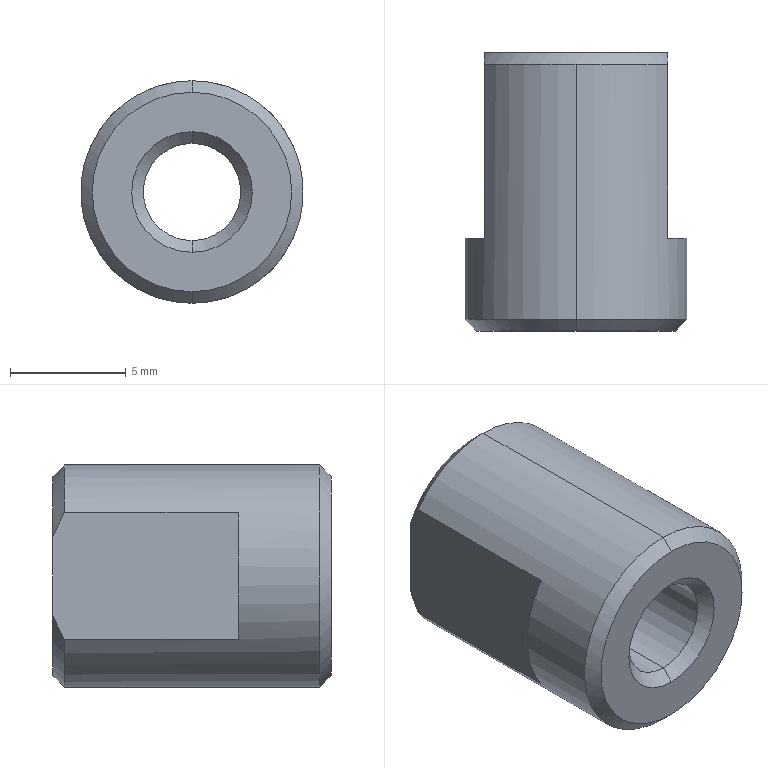Part | SolidWorks | features HoleWzd 1, ICE 1, Revolution 1 | 1 solid | 19 faces | box 9.6 x 12 x 9.6 mm | volume 642.366 mm3 | cone 9 | plane 6 | cylinder 4 | commonest cylinder face diameters 4.2 x2 9.6 x2
STEP:
#1=CARTESIAN_POINT('',(0.,11.5,-2.1));
#2=VERTEX_POINT('',#1);
#3=CARTESIAN_POINT('',(0.,11.5,2.1));
#4=VERTEX_POINT('',#3);
#5=CARTESIAN_POINT('',(0.,11.5,0.));
#6=DIRECTION('',(0.,1.,0.));
#7=DIRECTION('',(0.,0.,1.));
#8=AXIS2_PLACEMENT_3D('',#5,#6,#7);
#9=CIRCLE('',#8,2.1);
#10=EDGE_CURVE('',#2,#4,#9,.T.);
#11=ORIENTED_EDGE('',*,*,#10,.F.);
#12=CARTESIAN_POINT('',(0.,12.,-2.6));
#13=VERTEX_POINT('',#12);
#14=CARTESIAN_POINT('',(0.,12.,-2.6));
#15=DIRECTION('',(0.,0.7071,-0.7071));
#16=VECTOR('',#15,1000.);
#17=LINE('',#14,#16);
#18=EDGE_CURVE('',#2,#13,#17,.T.);
#19=ORIENTED_EDGE('',*,*,#18,.T.);
#20=CARTESIAN_POINT('',(0.,12.,2.6));
#21=VERTEX_POINT('',#20);
#22=CARTESIAN_POINT('',(0.,12.,0.));
#23=DIRECTION('',(0.,1.,0.));
#24=DIRECTION('',(0.,0.,1.));
#25=AXIS2_PLACEMENT_3D('',#22,#23,#24);
#26=CIRCLE('',#25,2.6);
#27=EDGE_CURVE('',#13,#21,#26,.T.);
#28=ORIENTED_EDGE('',*,*,#27,.T.);
#29=CARTESIAN_POINT('',(0.,12.,2.6));
#30=DIRECTION('',(0.,0.7071,0.7071));
#31=VECTOR('',#30,1000.);
#32=LINE('',#29,#31);
#33=EDGE_CURVE('',#4,#21,#32,.T.);
#34=ORIENTED_EDGE('',*,*,#33,.F.);
#35=EDGE_LOOP('',(#11,#19,#28,#34));
#36=FACE_OUTER_BOUND('',#35,.T.);
#37=CARTESIAN_POINT('',(0.,12.,0.));
#38=DIRECTION('',(0.,1.,0.));
#39=DIRECTION('',(0.,0.,1.));
#40=AXIS2_PLACEMENT_3D('',#37,#38,#39);
#41=CONICAL_SURFACE('',#40,2.6,0.7854);
#42=ADVANCED_FACE('',(#36),#41,.F.);
#43=CARTESIAN_POINT('',(0.,0.5,-2.1));
#44=VERTEX_POINT('',#43);
#45=CARTESIAN_POINT('',(0.,0.5,2.1));
#46=VERTEX_POINT('',#45);
#47=CARTESIAN_POINT('',(0.,0.5,0.));
#48=DIRECTION('',(0.,1.,0.));
#49=DIRECTION('',(0.,0.,1.));
#50=AXIS2_PLACEMENT_3D('',#47,#48,#49);
#51=CIRCLE('',#50,2.1);
#52=EDGE_CURVE('',#44,#46,#51,.T.);
#53=ORIENTED_EDGE('',*,*,#52,.F.);
#54=CARTESIAN_POINT('',(0.,12.,-2.1));
#55=DIRECTION('',(0.,1.,0.));
#56=VECTOR('',#55,1000.);
#57=LINE('',#54,#56);
#58=EDGE_CURVE('',#44,#2,#57,.T.);
#59=ORIENTED_EDGE('',*,*,#58,.T.);
#60=ORIENTED_EDGE('',*,*,#10,.T.);
#61=CARTESIAN_POINT('',(0.,12.,2.1));
#62=DIRECTION('',(0.,1.,0.));
#63=VECTOR('',#62,1000.);
#64=LINE('',#61,#63);
#65=EDGE_CURVE('',#46,#4,#64,.T.);
#66=ORIENTED_EDGE('',*,*,#65,.F.);
#67=EDGE_LOOP('',(#53,#59,#60,#66));
#68=FACE_OUTER_BOUND('',#67,.T.);
#69=CARTESIAN_POINT('',(0.,12.,0.));
#70=DIRECTION('',(0.,1.,0.));
#71=DIRECTION('',(0.,0.,1.));
#72=AXIS2_PLACEMENT_3D('',#69,#70,#71);
#73=CYLINDRICAL_SURFACE('',#72,2.1);
#74=ADVANCED_FACE('',(#68),#73,.F.);
#75=ORIENTED_EDGE('',*,*,#52,.T.);
#76=CARTESIAN_POINT('',(0.,0.,2.6));
#77=VERTEX_POINT('',#76);
#78=CARTESIAN_POINT('',(0.,0.5,2.1));
#79=DIRECTION('',(0.,-0.7071,0.7071));
#80=VECTOR('',#79,1000.);
#81=LINE('',#78,#80);
#82=EDGE_CURVE('',#46,#77,#81,.T.);
#83=ORIENTED_EDGE('',*,*,#82,.T.);
#84=CARTESIAN_POINT('',(0.,0.,-2.6));
#85=VERTEX_POINT('',#84);
#86=CARTESIAN_POINT('',(0.,0.,0.));
#87=DIRECTION('',(0.,1.,0.));
#88=DIRECTION('',(0.,0.,1.));
#89=AXIS2_PLACEMENT_3D('',#86,#87,#88);
#90=CIRCLE('',#89,2.6);
#91=EDGE_CURVE('',#85,#77,#90,.T.);
#92=ORIENTED_EDGE('',*,*,#91,.F.);
#93=CARTESIAN_POINT('',(0.,0.5,-2.1));
#94=DIRECTION('',(0.,-0.7071,-0.7071));
#95=VECTOR('',#94,1000.);
#96=LINE('',#93,#95);
#97=EDGE_CURVE('',#44,#85,#96,.T.);
#98=ORIENTED_EDGE('',*,*,#97,.F.);
#99=EDGE_LOOP('',(#75,#83,#92,#98));
#100=FACE_OUTER_BOUND('',#99,.T.);
#101=CARTESIAN_POINT('',(0.,0.5,0.));
#102=DIRECTION('',(0.,-1.,0.));
#103=DIRECTION('',(0.,0.,-1.));
#104=AXIS2_PLACEMENT_3D('',#101,#102,#103);
#105=CONICAL_SURFACE('',#104,2.1,0.7854);
#106=ADVANCED_FACE('',(#100),#105,.F.);
#107=CARTESIAN_POINT('',(0.,0.,-4.3));
#108=VERTEX_POINT('',#107);
#109=CARTESIAN_POINT('',(0.,0.,4.3));
#110=VERTEX_POINT('',#109);
#111=CARTESIAN_POINT('',(0.,0.,0.));
#112=DIRECTION('',(0.,-1.,0.));
#113=DIRECTION('',(0.,0.,-1.));
#114=AXIS2_PLACEMENT_3D('',#111,#112,#113);
#115=CIRCLE('',#114,4.3);
#116=EDGE_CURVE('',#108,#110,#115,.T.);
#117=ORIENTED_EDGE('',*,*,#116,.F.);
#118=CARTESIAN_POINT('',(0.,0.5,-4.8));
#119=VERTEX_POINT('',#118);
#120=CARTESIAN_POINT('',(0.,0.,-4.3));
#121=DIRECTION('',(0.,0.7071,-0.7071));
#122=VECTOR('',#121,1000.);
#123=LINE('',#120,#122);
#124=EDGE_CURVE('',#108,#119,#123,.T.);
#125=ORIENTED_EDGE('',*,*,#124,.T.);
#126=CARTESIAN_POINT('',(0.,0.5,4.8));
#127=VERTEX_POINT('',#126);
#128=CARTESIAN_POINT('',(0.,0.5,0.));
#129=DIRECTION('',(0.,-1.,0.));
#130=DIRECTION('',(0.,0.,-1.));
#131=AXIS2_PLACEMENT_3D('',#128,#129,#130);
#132=CIRCLE('',#131,4.8);
#133=EDGE_CURVE('',#119,#127,#132,.T.);
#134=ORIENTED_EDGE('',*,*,#133,.T.);
#135=CARTESIAN_POINT('',(0.,0.,4.3));
#136=DIRECTION('',(0.,0.7071,0.7071));
#137=VECTOR('',#136,1000.);
#138=LINE('',#135,#137);
#139=EDGE_CURVE('',#110,#127,#138,.T.);
#140=ORIENTED_EDGE('',*,*,#139,.F.);
#141=EDGE_LOOP('',(#117,#125,#134,#140));
#142=FACE_OUTER_BOUND('',#141,.T.);
#143=CARTESIAN_POINT('',(0.,0.,0.));
#144=DIRECTION('',(0.,1.,0.));
#145=DIRECTION('',(0.,0.,1.));
#146=AXIS2_PLACEMENT_3D('',#143,#144,#145);
#147=CONICAL_SURFACE('',#146,4.3,0.7854);
#148=ADVANCED_FACE('',(#142),#147,.T.);
#149=CARTESIAN_POINT('',(3.95,11.5,2.727));
#150=VERTEX_POINT('',#149);
#151=CARTESIAN_POINT('',(0.,11.5,4.8));
#152=VERTEX_POINT('',#151);
#153=CARTESIAN_POINT('',(0.,11.5,0.));
#154=DIRECTION('',(0.,-1.,0.));
#155=DIRECTION('',(0.,0.,-1.));
#156=AXIS2_PLACEMENT_3D('',#153,#154,#155);
#157=CIRCLE('',#156,4.8);
#158=EDGE_CURVE('',#150,#152,#157,.T.);
#159=ORIENTED_EDGE('',*,*,#158,.T.);
#160=CARTESIAN_POINT('',(0.,12.,4.8));
#161=DIRECTION('',(0.,-1.,0.));
#162=VECTOR('',#161,1000.);
#163=LINE('',#160,#162);
#164=EDGE_CURVE('',#152,#127,#163,.T.);
#165=ORIENTED_EDGE('',*,*,#164,.T.);
#166=ORIENTED_EDGE('',*,*,#133,.F.);
#167=CARTESIAN_POINT('',(0.,11.5,-4.8));
#168=VERTEX_POINT('',#167);
#169=CARTESIAN_POINT('',(0.,12.,-4.8));
#170=DIRECTION('',(0.,-1.,0.));
#171=VECTOR('',#170,1000.);
#172=LINE('',#169,#171);
#173=EDGE_CURVE('',#168,#119,#172,.T.);
#174=ORIENTED_EDGE('',*,*,#173,.F.);
#175=CARTESIAN_POINT('',(3.95,11.5,-2.727));
#176=VERTEX_POINT('',#175);
#177=CARTESIAN_POINT('',(0.,11.5,0.));
#178=DIRECTION('',(0.,-1.,0.));
#179=DIRECTION('',(0.,0.,-1.));
#180=AXIS2_PLACEMENT_3D('',#177,#178,#179);
#181=CIRCLE('',#180,4.8);
#182=EDGE_CURVE('',#168,#176,#181,.T.);
#183=ORIENTED_EDGE('',*,*,#182,.T.);
#184=CARTESIAN_POINT('',(3.95,4.,-2.727));
#185=VERTEX_POINT('',#184);
#186=CARTESIAN_POINT('',(3.95,12.,-2.727));
#187=DIRECTION('',(0.,1.,0.));
#188=VECTOR('',#187,1000.);
#189=LINE('',#186,#188);
#190=EDGE_CURVE('',#185,#176,#189,.T.);
#191=ORIENTED_EDGE('',*,*,#190,.F.);
#192=CARTESIAN_POINT('',(3.95,4.,2.727));
#193=VERTEX_POINT('',#192);
#194=CARTESIAN_POINT('',(0.,4.,0.));
#195=DIRECTION('',(0.,1.,0.));
#196=DIRECTION('',(0.,0.,-1.));
#197=AXIS2_PLACEMENT_3D('',#194,#195,#196);
#198=CIRCLE('',#197,4.8);
#199=EDGE_CURVE('',#193,#185,#198,.T.);
#200=ORIENTED_EDGE('',*,*,#199,.F.);
#201=CARTESIAN_POINT('',(3.95,12.,2.727));
#202=DIRECTION('',(0.,-1.,0.));
#203=VECTOR('',#202,1000.);
#204=LINE('',#201,#203);
#205=EDGE_CURVE('',#150,#193,#204,.T.);
#206=ORIENTED_EDGE('',*,*,#205,.F.);
#207=EDGE_LOOP('',(#159,#165,#166,#174,#183,#191,#200,#206));
#208=FACE_OUTER_BOUND('',#207,.T.);
#209=CARTESIAN_POINT('',(0.,12.,0.));
#210=DIRECTION('',(0.,-1.,0.));
#211=DIRECTION('',(0.,0.,-1.));
#212=AXIS2_PLACEMENT_3D('',#209,#210,#211);
#213=CYLINDRICAL_SURFACE('',#212,4.8);
#214=ADVANCED_FACE('',(#208),#213,.T.);
#215=CARTESIAN_POINT('',(-3.95,12.,-1.699));
#216=VERTEX_POINT('',#215);
#217=CARTESIAN_POINT('',(0.,12.,-4.3));
#218=VERTEX_POINT('',#217);
#219=CARTESIAN_POINT('',(0.,12.,0.));
#220=DIRECTION('',(0.,-1.,0.));
#221=DIRECTION('',(0.,0.,-1.));
#222=AXIS2_PLACEMENT_3D('',#219,#220,#221);
#223=CIRCLE('',#222,4.3);
#224=EDGE_CURVE('',#216,#218,#223,.T.);
#225=ORIENTED_EDGE('',*,*,#224,.T.);
#226=CARTESIAN_POINT('',(0.,11.5,-4.8));
#227=DIRECTION('',(0.,-0.7071,-0.7071));
#228=VECTOR('',#227,1000.);
#229=LINE('',#226,#228);
#230=EDGE_CURVE('',#218,#168,#229,.T.);
#231=ORIENTED_EDGE('',*,*,#230,.T.);
#232=CARTESIAN_POINT('',(-3.95,11.5,-2.727));
#233=VERTEX_POINT('',#232);
#234=CARTESIAN_POINT('',(0.,11.5,0.));
#235=DIRECTION('',(0.,-1.,0.));
#236=DIRECTION('',(0.,0.,-1.));
#237=AXIS2_PLACEMENT_3D('',#234,#235,#236);
#238=CIRCLE('',#237,4.8);
#239=EDGE_CURVE('',#233,#168,#238,.T.);
#240=ORIENTED_EDGE('',*,*,#239,.F.);
#241=CARTESIAN_POINT('',(-3.95,12.,-1.699));
#242=CARTESIAN_POINT('',(-3.95,11.859,-2.056));
#243=CARTESIAN_POINT('',(-3.95,11.688,-2.397));
#244=CARTESIAN_POINT('',(-3.95,11.5,-2.727));
#245=B_SPLINE_CURVE_WITH_KNOTS('',3,(#241,#242,#243,#244),.UNSPECIFIED.,.F.,.F.,(4,4),(0.01378,0.01493),.UNSPECIFIED.);
#246=EDGE_CURVE('',#216,#233,#245,.T.);
#247=ORIENTED_EDGE('',*,*,#246,.F.);
#248=EDGE_LOOP('',(#225,#231,#240,#247));
#249=FACE_OUTER_BOUND('',#248,.T.);
#250=CARTESIAN_POINT('',(0.,11.5,0.));
#251=DIRECTION('',(0.,-1.,0.));
#252=DIRECTION('',(0.,0.,-1.));
#253=AXIS2_PLACEMENT_3D('',#250,#251,#252);
#254=CONICAL_SURFACE('',#253,4.8,0.7854);
#255=ADVANCED_FACE('',(#249),#254,.T.);
#256=CARTESIAN_POINT('',(-3.95,11.5,2.727));
#257=VERTEX_POINT('',#256);
#258=CARTESIAN_POINT('',(-3.95,12.,1.699));
#259=VERTEX_POINT('',#258);
#260=CARTESIAN_POINT('',(-3.95,11.5,2.727));
#261=CARTESIAN_POINT('',(-3.95,11.689,2.395));
#262=CARTESIAN_POINT('',(-3.95,11.86,2.055));
#263=CARTESIAN_POINT('',(-3.95,12.,1.699));
#264=B_SPLINE_CURVE_WITH_KNOTS('',3,(#260,#261,#262,#263),.UNSPECIFIED.,.F.,.F.,(4,4),(0.009145,0.01029),.UNSPECIFIED.);
#265=EDGE_CURVE('',#257,#259,#264,.T.);
#266=ORIENTED_EDGE('',*,*,#265,.F.);
#267=CARTESIAN_POINT('',(0.,11.5,0.));
#268=DIRECTION('',(0.,-1.,0.));
#269=DIRECTION('',(0.,0.,-1.));
#270=AXIS2_PLACEMENT_3D('',#267,#268,#269);
#271=CIRCLE('',#270,4.8);
#272=EDGE_CURVE('',#152,#257,#271,.T.);
#273=ORIENTED_EDGE('',*,*,#272,.F.);
#274=ORIENTED_EDGE('',*,*,#158,.F.);
#275=CARTESIAN_POINT('',(3.95,12.,1.699));
#276=VERTEX_POINT('',#275);
#277=CARTESIAN_POINT('',(3.95,12.,1.699));
#278=CARTESIAN_POINT('',(3.95,11.859,2.056));
#279=CARTESIAN_POINT('',(3.95,11.688,2.397));
#280=CARTESIAN_POINT('',(3.95,11.5,2.727));
#281=B_SPLINE_CURVE_WITH_KNOTS('',3,(#277,#278,#279,#280),.UNSPECIFIED.,.F.,.F.,(4,4),(0.01378,0.01493),.UNSPECIFIED.);
#282=EDGE_CURVE('',#276,#150,#281,.T.);
#283=ORIENTED_EDGE('',*,*,#282,.F.);
#284=CARTESIAN_POINT('',(0.,12.,0.));
#285=DIRECTION('',(0.,-1.,0.));
#286=DIRECTION('',(0.,0.,-1.));
#287=AXIS2_PLACEMENT_3D('',#284,#285,#286);
#288=CIRCLE('',#287,4.3);
#289=EDGE_CURVE('',#276,#259,#288,.T.);
#290=ORIENTED_EDGE('',*,*,#289,.T.);
#291=EDGE_LOOP('',(#266,#273,#274,#283,#290));
#292=FACE_OUTER_BOUND('',#291,.T.);
#293=CARTESIAN_POINT('',(0.,11.5,0.));
#294=DIRECTION('',(0.,-1.,0.));
#295=DIRECTION('',(0.,0.,-1.));
#296=AXIS2_PLACEMENT_3D('',#293,#294,#295);
#297=CONICAL_SURFACE('',#296,4.8,0.7854);
#298=ADVANCED_FACE('',(#292),#297,.T.);
#299=CARTESIAN_POINT('',(-3.95,12.,-5.));
#300=DIRECTION('',(0.,0.,1.));
#301=VECTOR('',#300,1000.);
#302=LINE('',#299,#301);
#303=EDGE_CURVE('',#216,#259,#302,.T.);
#304=ORIENTED_EDGE('',*,*,#303,.T.);
#305=ORIENTED_EDGE('',*,*,#289,.F.);
#306=CARTESIAN_POINT('',(3.95,12.,-1.699));
#307=VERTEX_POINT('',#306);
#308=CARTESIAN_POINT('',(3.95,12.,-5.));
#309=DIRECTION('',(0.,0.,1.));
#310=VECTOR('',#309,1000.);
#311=LINE('',#308,#310);
#312=EDGE_CURVE('',#307,#276,#311,.T.);
#313=ORIENTED_EDGE('',*,*,#312,.F.);
#314=CARTESIAN_POINT('',(0.,12.,0.));
#315=DIRECTION('',(0.,-1.,0.));
#316=DIRECTION('',(0.,0.,-1.));
#317=AXIS2_PLACEMENT_3D('',#314,#315,#316);
#318=CIRCLE('',#317,4.3);
#319=EDGE_CURVE('',#218,#307,#318,.T.);
#320=ORIENTED_EDGE('',*,*,#319,.F.);
#321=ORIENTED_EDGE('',*,*,#224,.F.);
#322=EDGE_LOOP('',(#304,#305,#313,#320,#321));
#323=FACE_OUTER_BOUND('',#322,.T.);
#324=CARTESIAN_POINT('',(0.,12.,0.));
#325=DIRECTION('',(0.,1.,0.));
#326=DIRECTION('',(0.,0.,1.));
#327=AXIS2_PLACEMENT_3D('',#324,#325,#326);
#328=CIRCLE('',#327,2.6);
#329=EDGE_CURVE('',#21,#13,#328,.T.);
#330=ORIENTED_EDGE('',*,*,#329,.F.);
#331=ORIENTED_EDGE('',*,*,#27,.F.);
#332=EDGE_LOOP('',(#330,#331));
#333=FACE_BOUND('',#332,.T.);
#334=CARTESIAN_POINT('',(0.,12.,0.));
#335=DIRECTION('',(0.,1.,0.));
#336=DIRECTION('',(0.,0.,1.));
#337=AXIS2_PLACEMENT_3D('',#334,#335,#336);
#338=PLANE('',#337);
#339=ADVANCED_FACE('',(#323,#333),#338,.T.);
#340=ORIENTED_EDGE('',*,*,#230,.F.);
#341=ORIENTED_EDGE('',*,*,#319,.T.);
#342=CARTESIAN_POINT('',(3.95,11.5,-2.727));
#343=CARTESIAN_POINT('',(3.95,11.689,-2.395));
#344=CARTESIAN_POINT('',(3.95,11.86,-2.055));
#345=CARTESIAN_POINT('',(3.95,12.,-1.699));
#346=B_SPLINE_CURVE_WITH_KNOTS('',3,(#342,#343,#344,#345),.UNSPECIFIED.,.F.,.F.,(4,4),(0.009145,0.01029),.UNSPECIFIED.);
#347=EDGE_CURVE('',#176,#307,#346,.T.);
#348=ORIENTED_EDGE('',*,*,#347,.F.);
#349=ORIENTED_EDGE('',*,*,#182,.F.);
#350=EDGE_LOOP('',(#340,#341,#348,#349));
#351=FACE_OUTER_BOUND('',#350,.T.);
#352=CARTESIAN_POINT('',(0.,11.5,0.));
#353=DIRECTION('',(0.,-1.,0.));
#354=DIRECTION('',(0.,0.,-1.));
#355=AXIS2_PLACEMENT_3D('',#352,#353,#354);
#356=CONICAL_SURFACE('',#355,4.8,0.7854);
#357=ADVANCED_FACE('',(#351),#356,.T.);
#358=ORIENTED_EDGE('',*,*,#164,.F.);
#359=ORIENTED_EDGE('',*,*,#272,.T.);
#360=CARTESIAN_POINT('',(-3.95,4.,2.727));
#361=VERTEX_POINT('',#360);
#362=CARTESIAN_POINT('',(-3.95,12.,2.727));
#363=DIRECTION('',(0.,1.,0.));
#364=VECTOR('',#363,1000.);
#365=LINE('',#362,#364);
#366=EDGE_CURVE('',#361,#257,#365,.T.);
#367=ORIENTED_EDGE('',*,*,#366,.F.);
#368=CARTESIAN_POINT('',(-3.95,4.,-2.727));
#369=VERTEX_POINT('',#368);
#370=CARTESIAN_POINT('',(0.,4.,0.));
#371=DIRECTION('',(0.,1.,0.));
#372=DIRECTION('',(0.,0.,-1.));
#373=AXIS2_PLACEMENT_3D('',#370,#371,#372);
#374=CIRCLE('',#373,4.8);
#375=EDGE_CURVE('',#369,#361,#374,.T.);
#376=ORIENTED_EDGE('',*,*,#375,.F.);
#377=CARTESIAN_POINT('',(-3.95,12.,-2.727));
#378=DIRECTION('',(0.,-1.,0.));
#379=VECTOR('',#378,1000.);
#380=LINE('',#377,#379);
#381=EDGE_CURVE('',#233,#369,#380,.T.);
#382=ORIENTED_EDGE('',*,*,#381,.F.);
#383=ORIENTED_EDGE('',*,*,#239,.T.);
#384=ORIENTED_EDGE('',*,*,#173,.T.);
#385=CARTESIAN_POINT('',(0.,0.5,0.));
#386=DIRECTION('',(0.,-1.,0.));
#387=DIRECTION('',(0.,0.,-1.));
#388=AXIS2_PLACEMENT_3D('',#385,#386,#387);
#389=CIRCLE('',#388,4.8);
#390=EDGE_CURVE('',#127,#119,#389,.T.);
#391=ORIENTED_EDGE('',*,*,#390,.F.);
#392=EDGE_LOOP('',(#358,#359,#367,#376,#382,#383,#384,#391));
#393=FACE_OUTER_BOUND('',#392,.T.);
#394=CARTESIAN_POINT('',(0.,12.,0.));
#395=DIRECTION('',(0.,-1.,0.));
#396=DIRECTION('',(0.,0.,-1.));
#397=AXIS2_PLACEMENT_3D('',#394,#395,#396);
#398=CYLINDRICAL_SURFACE('',#397,4.8);
#399=ADVANCED_FACE('',(#393),#398,.T.);
#400=ORIENTED_EDGE('',*,*,#124,.F.);
#401=CARTESIAN_POINT('',(0.,0.,0.));
#402=DIRECTION('',(0.,-1.,0.));
#403=DIRECTION('',(0.,0.,-1.));
#404=AXIS2_PLACEMENT_3D('',#401,#402,#403);
#405=CIRCLE('',#404,4.3);
#406=EDGE_CURVE('',#110,#108,#405,.T.);
#407=ORIENTED_EDGE('',*,*,#406,.F.);
#408=ORIENTED_EDGE('',*,*,#139,.T.);
#409=ORIENTED_EDGE('',*,*,#390,.T.);
#410=EDGE_LOOP('',(#400,#407,#408,#409));
#411=FACE_OUTER_BOUND('',#410,.T.);
#412=CARTESIAN_POINT('',(0.,0.,0.));
#413=DIRECTION('',(0.,1.,0.));
#414=DIRECTION('',(0.,0.,1.));
#415=AXIS2_PLACEMENT_3D('',#412,#413,#414);
#416=CONICAL_SURFACE('',#415,4.3,0.7854);
#417=ADVANCED_FACE('',(#411),#416,.T.);
#418=ORIENTED_EDGE('',*,*,#91,.T.);
#419=CARTESIAN_POINT('',(0.,0.,0.));
#420=DIRECTION('',(0.,1.,0.));
#421=DIRECTION('',(0.,0.,1.));
#422=AXIS2_PLACEMENT_3D('',#419,#420,#421);
#423=CIRCLE('',#422,2.6);
#424=EDGE_CURVE('',#77,#85,#423,.T.);
#425=ORIENTED_EDGE('',*,*,#424,.T.);
#426=EDGE_LOOP('',(#418,#425));
#427=FACE_BOUND('',#426,.T.);
#428=ORIENTED_EDGE('',*,*,#406,.T.);
#429=ORIENTED_EDGE('',*,*,#116,.T.);
#430=EDGE_LOOP('',(#428,#429));
#431=FACE_OUTER_BOUND('',#430,.T.);
#432=CARTESIAN_POINT('',(0.,0.,0.));
#433=DIRECTION('',(0.,-1.,0.));
#434=DIRECTION('',(0.,0.,-1.));
#435=AXIS2_PLACEMENT_3D('',#432,#433,#434);
#436=PLANE('',#435);
#437=ADVANCED_FACE('',(#427,#431),#436,.T.);
#438=ORIENTED_EDGE('',*,*,#82,.F.);
#439=CARTESIAN_POINT('',(0.,0.5,0.));
#440=DIRECTION('',(0.,1.,0.));
#441=DIRECTION('',(0.,0.,1.));
#442=AXIS2_PLACEMENT_3D('',#439,#440,#441);
#443=CIRCLE('',#442,2.1);
#444=EDGE_CURVE('',#46,#44,#443,.T.);
#445=ORIENTED_EDGE('',*,*,#444,.T.);
#446=ORIENTED_EDGE('',*,*,#97,.T.);
#447=ORIENTED_EDGE('',*,*,#424,.F.);
#448=EDGE_LOOP('',(#438,#445,#446,#447));
#449=FACE_OUTER_BOUND('',#448,.T.);
#450=CARTESIAN_POINT('',(0.,0.5,0.));
#451=DIRECTION('',(0.,-1.,0.));
#452=DIRECTION('',(0.,0.,-1.));
#453=AXIS2_PLACEMENT_3D('',#450,#451,#452);
#454=CONICAL_SURFACE('',#453,2.1,0.7854);
#455=ADVANCED_FACE('',(#449),#454,.F.);
#456=ORIENTED_EDGE('',*,*,#58,.F.);
#457=ORIENTED_EDGE('',*,*,#444,.F.);
#458=ORIENTED_EDGE('',*,*,#65,.T.);
#459=CARTESIAN_POINT('',(0.,11.5,0.));
#460=DIRECTION('',(0.,1.,0.));
#461=DIRECTION('',(0.,0.,1.));
#462=AXIS2_PLACEMENT_3D('',#459,#460,#461);
#463=CIRCLE('',#462,2.1);
#464=EDGE_CURVE('',#4,#2,#463,.T.);
#465=ORIENTED_EDGE('',*,*,#464,.T.);
#466=EDGE_LOOP('',(#456,#457,#458,#465));
#467=FACE_OUTER_BOUND('',#466,.T.);
#468=CARTESIAN_POINT('',(0.,12.,0.));
#469=DIRECTION('',(0.,1.,0.));
#470=DIRECTION('',(0.,0.,1.));
#471=AXIS2_PLACEMENT_3D('',#468,#469,#470);
#472=CYLINDRICAL_SURFACE('',#471,2.1);
#473=ADVANCED_FACE('',(#467),#472,.F.);
#474=ORIENTED_EDGE('',*,*,#18,.F.);
#475=ORIENTED_EDGE('',*,*,#464,.F.);
#476=ORIENTED_EDGE('',*,*,#33,.T.);
#477=ORIENTED_EDGE('',*,*,#329,.T.);
#478=EDGE_LOOP('',(#474,#475,#476,#477));
#479=FACE_OUTER_BOUND('',#478,.T.);
#480=CARTESIAN_POINT('',(0.,12.,0.));
#481=DIRECTION('',(0.,1.,0.));
#482=DIRECTION('',(0.,0.,1.));
#483=AXIS2_PLACEMENT_3D('',#480,#481,#482);
#484=CONICAL_SURFACE('',#483,2.6,0.7854);
#485=ADVANCED_FACE('',(#479),#484,.F.);
#486=ORIENTED_EDGE('',*,*,#199,.T.);
#487=CARTESIAN_POINT('',(3.95,4.,-5.));
#488=DIRECTION('',(0.,0.,1.));
#489=VECTOR('',#488,1000.);
#490=LINE('',#487,#489);
#491=EDGE_CURVE('',#185,#193,#490,.T.);
#492=ORIENTED_EDGE('',*,*,#491,.T.);
#493=EDGE_LOOP('',(#486,#492));
#494=FACE_OUTER_BOUND('',#493,.T.);
#495=CARTESIAN_POINT('',(5.334,4.,-5.));
#496=DIRECTION('',(0.,-1.,0.));
#497=DIRECTION('',(0.,0.,-1.));
#498=AXIS2_PLACEMENT_3D('',#495,#496,#497);
#499=PLANE('',#498);
#500=ADVANCED_FACE('',(#494),#499,.F.);
#501=ORIENTED_EDGE('',*,*,#347,.T.);
#502=ORIENTED_EDGE('',*,*,#312,.T.);
#503=ORIENTED_EDGE('',*,*,#282,.T.);
#504=ORIENTED_EDGE('',*,*,#205,.T.);
#505=ORIENTED_EDGE('',*,*,#491,.F.);
#506=ORIENTED_EDGE('',*,*,#190,.T.);
#507=EDGE_LOOP('',(#501,#502,#503,#504,#505,#506));
#508=FACE_OUTER_BOUND('',#507,.T.);
#509=CARTESIAN_POINT('',(3.95,12.,-5.));
#510=DIRECTION('',(-1.,0.,0.));
#511=DIRECTION('',(0.,-1.,0.));
#512=AXIS2_PLACEMENT_3D('',#509,#510,#511);
#513=PLANE('',#512);
#514=ADVANCED_FACE('',(#508),#513,.F.);
#515=ORIENTED_EDGE('',*,*,#265,.T.);
#516=ORIENTED_EDGE('',*,*,#303,.F.);
#517=ORIENTED_EDGE('',*,*,#246,.T.);
#518=ORIENTED_EDGE('',*,*,#381,.T.);
#519=CARTESIAN_POINT('',(-3.95,4.,-5.));
#520=DIRECTION('',(0.,0.,1.));
#521=VECTOR('',#520,1000.);
#522=LINE('',#519,#521);
#523=EDGE_CURVE('',#369,#361,#522,.T.);
#524=ORIENTED_EDGE('',*,*,#523,.T.);
#525=ORIENTED_EDGE('',*,*,#366,.T.);
#526=EDGE_LOOP('',(#515,#516,#517,#518,#524,#525));
#527=FACE_OUTER_BOUND('',#526,.T.);
#528=CARTESIAN_POINT('',(-3.95,12.,-5.));
#529=DIRECTION('',(1.,0.,0.));
#530=DIRECTION('',(0.,1.,0.));
#531=AXIS2_PLACEMENT_3D('',#528,#529,#530);
#532=PLANE('',#531);
#533=ADVANCED_FACE('',(#527),#532,.F.);
#534=ORIENTED_EDGE('',*,*,#375,.T.);
#535=ORIENTED_EDGE('',*,*,#523,.F.);
#536=EDGE_LOOP('',(#534,#535));
#537=FACE_OUTER_BOUND('',#536,.T.);
#538=CARTESIAN_POINT('',(-5.334,4.,-5.));
#539=DIRECTION('',(0.,-1.,0.));
#540=DIRECTION('',(0.,0.,-1.));
#541=AXIS2_PLACEMENT_3D('',#538,#539,#540);
#542=PLANE('',#541);
#543=ADVANCED_FACE('',(#537),#542,.F.);
#544=CLOSED_SHELL('',(#42,#74,#106,#148,#214,#255,#298,#339,#357,#399,#417,#437,#455,#473,#485,#500,#514,#533,#543));
#545=MANIFOLD_SOLID_BREP('',#544);
#546=CARTESIAN_POINT('',(0.,0.,0.));
#547=DIRECTION('',(0.,0.,1.));
#548=DIRECTION('',(1.,0.,0.));
#549=AXIS2_PLACEMENT_3D('',#546,#547,#548);
#550=(LENGTH_UNIT()NAMED_UNIT(*)SI_UNIT(.MILLI.,.METRE.));
#551=UNCERTAINTY_MEASURE_WITH_UNIT(LENGTH_MEASURE(0.00001),#550,'','');
#552=(NAMED_UNIT(*)PLANE_ANGLE_UNIT()SI_UNIT($,.RADIAN.));
#553=(NAMED_UNIT(*)SI_UNIT($,.STERADIAN.)SOLID_ANGLE_UNIT());
#554=(GEOMETRIC_REPRESENTATION_CONTEXT(3)GLOBAL_UNCERTAINTY_ASSIGNED_CONTEXT((#551))GLOBAL_UNIT_ASSIGNED_CONTEXT((#550,#552,#553))REPRESENTATION_CONTEXT('',''));
#555=ADVANCED_BREP_SHAPE_REPRESENTATION('',(#545,#549),#554);